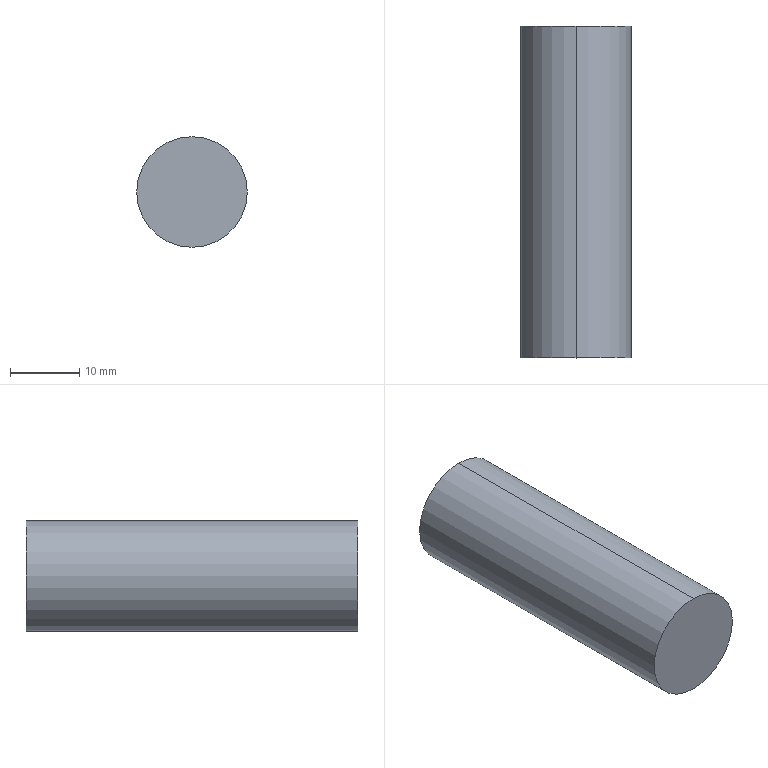Part | SolidWorks | features Extrusion 1, HoleWzd 1 | 1 solid | 8 faces | box 16 x 48 x 16 mm | volume 8682 mm3 | cylinder 4 | cone 2 | plane 2 | commonest cylinder face diameters 6.8 x2 16 x2
STEP:
#1=CARTESIAN_POINT('',(0.,22.,-3.4));
#2=VERTEX_POINT('',#1);
#3=CARTESIAN_POINT('',(0.,22.,3.4));
#4=VERTEX_POINT('',#3);
#5=CARTESIAN_POINT('',(0.,22.,0.));
#6=DIRECTION('',(0.,1.,0.));
#7=DIRECTION('',(0.,0.,1.));
#8=AXIS2_PLACEMENT_3D('',#5,#6,#7);
#9=CIRCLE('',#8,3.4);
#10=EDGE_CURVE('',#2,#4,#9,.T.);
#11=ORIENTED_EDGE('',*,*,#10,.F.);
#12=CARTESIAN_POINT('',(0.,48.,-3.4));
#13=VERTEX_POINT('',#12);
#14=CARTESIAN_POINT('',(0.,48.,-3.4));
#15=DIRECTION('',(0.,1.,0.));
#16=VECTOR('',#15,1000.);
#17=LINE('',#14,#16);
#18=EDGE_CURVE('',#2,#13,#17,.T.);
#19=ORIENTED_EDGE('',*,*,#18,.T.);
#20=CARTESIAN_POINT('',(0.,48.,3.4));
#21=VERTEX_POINT('',#20);
#22=CARTESIAN_POINT('',(0.,48.,0.));
#23=DIRECTION('',(0.,1.,0.));
#24=DIRECTION('',(0.,0.,1.));
#25=AXIS2_PLACEMENT_3D('',#22,#23,#24);
#26=CIRCLE('',#25,3.4);
#27=EDGE_CURVE('',#13,#21,#26,.T.);
#28=ORIENTED_EDGE('',*,*,#27,.T.);
#29=CARTESIAN_POINT('',(0.,48.,3.4));
#30=DIRECTION('',(0.,1.,0.));
#31=VECTOR('',#30,1000.);
#32=LINE('',#29,#31);
#33=EDGE_CURVE('',#4,#21,#32,.T.);
#34=ORIENTED_EDGE('',*,*,#33,.F.);
#35=EDGE_LOOP('',(#11,#19,#28,#34));
#36=FACE_OUTER_BOUND('',#35,.T.);
#37=CARTESIAN_POINT('',(0.,48.,0.));
#38=DIRECTION('',(0.,1.,0.));
#39=DIRECTION('',(0.,0.,1.));
#40=AXIS2_PLACEMENT_3D('',#37,#38,#39);
#41=CYLINDRICAL_SURFACE('',#40,3.4);
#42=ADVANCED_FACE('',(#36),#41,.F.);
#43=CARTESIAN_POINT('',(0.,19.957,0.));
#44=VERTEX_POINT('',#43);
#45=CARTESIAN_POINT('',(0.,22.,3.4));
#46=DIRECTION('',(0.,0.515,0.8572));
#47=VECTOR('',#46,1000.);
#48=LINE('',#45,#47);
#49=EDGE_CURVE('',#44,#4,#48,.T.);
#50=ORIENTED_EDGE('',*,*,#49,.F.);
#51=CARTESIAN_POINT('',(0.,22.,-3.4));
#52=DIRECTION('',(0.,0.515,-0.8572));
#53=VECTOR('',#52,1000.);
#54=LINE('',#51,#53);
#55=EDGE_CURVE('',#44,#2,#54,.T.);
#56=ORIENTED_EDGE('',*,*,#55,.T.);
#57=ORIENTED_EDGE('',*,*,#10,.T.);
#58=EDGE_LOOP('',(#50,#56,#57));
#59=FACE_OUTER_BOUND('',#58,.T.);
#60=CARTESIAN_POINT('',(0.,22.,0.));
#61=DIRECTION('',(0.,1.,0.));
#62=DIRECTION('',(0.,0.,1.));
#63=AXIS2_PLACEMENT_3D('',#60,#61,#62);
#64=CONICAL_SURFACE('',#63,3.4,1.03);
#65=ADVANCED_FACE('',(#59),#64,.F.);
#66=CARTESIAN_POINT('',(0.,48.,8.));
#67=VERTEX_POINT('',#66);
#68=CARTESIAN_POINT('',(0.,48.,-8.));
#69=VERTEX_POINT('',#68);
#70=CARTESIAN_POINT('',(0.,48.,0.));
#71=DIRECTION('',(0.,1.,0.));
#72=DIRECTION('',(0.,0.,1.));
#73=AXIS2_PLACEMENT_3D('',#70,#71,#72);
#74=CIRCLE('',#73,8.);
#75=EDGE_CURVE('',#67,#69,#74,.T.);
#76=ORIENTED_EDGE('',*,*,#75,.F.);
#77=CARTESIAN_POINT('',(0.,0.,8.));
#78=VERTEX_POINT('',#77);
#79=CARTESIAN_POINT('',(0.,48.,8.));
#80=DIRECTION('',(0.,-1.,0.));
#81=VECTOR('',#80,1000.);
#82=LINE('',#79,#81);
#83=EDGE_CURVE('',#67,#78,#82,.T.);
#84=ORIENTED_EDGE('',*,*,#83,.T.);
#85=CARTESIAN_POINT('',(0.,0.,-8.));
#86=VERTEX_POINT('',#85);
#87=CARTESIAN_POINT('',(0.,0.,0.));
#88=DIRECTION('',(0.,1.,0.));
#89=DIRECTION('',(0.,0.,1.));
#90=AXIS2_PLACEMENT_3D('',#87,#88,#89);
#91=CIRCLE('',#90,8.);
#92=EDGE_CURVE('',#78,#86,#91,.T.);
#93=ORIENTED_EDGE('',*,*,#92,.T.);
#94=CARTESIAN_POINT('',(0.,48.,-8.));
#95=DIRECTION('',(0.,-1.,0.));
#96=VECTOR('',#95,1000.);
#97=LINE('',#94,#96);
#98=EDGE_CURVE('',#69,#86,#97,.T.);
#99=ORIENTED_EDGE('',*,*,#98,.F.);
#100=EDGE_LOOP('',(#76,#84,#93,#99));
#101=FACE_OUTER_BOUND('',#100,.T.);
#102=CARTESIAN_POINT('',(0.,48.,0.));
#103=DIRECTION('',(0.,-1.,0.));
#104=DIRECTION('',(0.,0.,-1.));
#105=AXIS2_PLACEMENT_3D('',#102,#103,#104);
#106=CYLINDRICAL_SURFACE('',#105,8.);
#107=ADVANCED_FACE('',(#101),#106,.T.);
#108=ORIENTED_EDGE('',*,*,#83,.F.);
#109=CARTESIAN_POINT('',(0.,48.,0.));
#110=DIRECTION('',(0.,1.,0.));
#111=DIRECTION('',(0.,0.,1.));
#112=AXIS2_PLACEMENT_3D('',#109,#110,#111);
#113=CIRCLE('',#112,8.);
#114=EDGE_CURVE('',#69,#67,#113,.T.);
#115=ORIENTED_EDGE('',*,*,#114,.F.);
#116=ORIENTED_EDGE('',*,*,#98,.T.);
#117=CARTESIAN_POINT('',(0.,0.,0.));
#118=DIRECTION('',(0.,1.,0.));
#119=DIRECTION('',(0.,0.,1.));
#120=AXIS2_PLACEMENT_3D('',#117,#118,#119);
#121=CIRCLE('',#120,8.);
#122=EDGE_CURVE('',#86,#78,#121,.T.);
#123=ORIENTED_EDGE('',*,*,#122,.T.);
#124=EDGE_LOOP('',(#108,#115,#116,#123));
#125=FACE_OUTER_BOUND('',#124,.T.);
#126=CARTESIAN_POINT('',(0.,48.,0.));
#127=DIRECTION('',(0.,-1.,0.));
#128=DIRECTION('',(0.,0.,-1.));
#129=AXIS2_PLACEMENT_3D('',#126,#127,#128);
#130=CYLINDRICAL_SURFACE('',#129,8.);
#131=ADVANCED_FACE('',(#125),#130,.T.);
#132=CARTESIAN_POINT('',(0.,48.,0.));
#133=DIRECTION('',(0.,1.,0.));
#134=DIRECTION('',(0.,0.,1.));
#135=AXIS2_PLACEMENT_3D('',#132,#133,#134);
#136=CIRCLE('',#135,3.4);
#137=EDGE_CURVE('',#21,#13,#136,.T.);
#138=ORIENTED_EDGE('',*,*,#137,.F.);
#139=ORIENTED_EDGE('',*,*,#27,.F.);
#140=EDGE_LOOP('',(#138,#139));
#141=FACE_BOUND('',#140,.T.);
#142=ORIENTED_EDGE('',*,*,#114,.T.);
#143=ORIENTED_EDGE('',*,*,#75,.T.);
#144=EDGE_LOOP('',(#142,#143));
#145=FACE_OUTER_BOUND('',#144,.T.);
#146=CARTESIAN_POINT('',(0.,48.,0.));
#147=DIRECTION('',(0.,1.,0.));
#148=DIRECTION('',(0.,0.,1.));
#149=AXIS2_PLACEMENT_3D('',#146,#147,#148);
#150=PLANE('',#149);
#151=ADVANCED_FACE('',(#141,#145),#150,.T.);
#152=ORIENTED_EDGE('',*,*,#122,.F.);
#153=ORIENTED_EDGE('',*,*,#92,.F.);
#154=EDGE_LOOP('',(#152,#153));
#155=FACE_OUTER_BOUND('',#154,.T.);
#156=CARTESIAN_POINT('',(0.,0.,0.));
#157=DIRECTION('',(0.,1.,0.));
#158=DIRECTION('',(0.,0.,1.));
#159=AXIS2_PLACEMENT_3D('',#156,#157,#158);
#160=PLANE('',#159);
#161=ADVANCED_FACE('',(#155),#160,.F.);
#162=ORIENTED_EDGE('',*,*,#55,.F.);
#163=ORIENTED_EDGE('',*,*,#49,.T.);
#164=CARTESIAN_POINT('',(0.,22.,0.));
#165=DIRECTION('',(0.,1.,0.));
#166=DIRECTION('',(0.,0.,1.));
#167=AXIS2_PLACEMENT_3D('',#164,#165,#166);
#168=CIRCLE('',#167,3.4);
#169=EDGE_CURVE('',#4,#2,#168,.T.);
#170=ORIENTED_EDGE('',*,*,#169,.T.);
#171=EDGE_LOOP('',(#162,#163,#170));
#172=FACE_OUTER_BOUND('',#171,.T.);
#173=CARTESIAN_POINT('',(0.,22.,0.));
#174=DIRECTION('',(0.,1.,0.));
#175=DIRECTION('',(0.,0.,1.));
#176=AXIS2_PLACEMENT_3D('',#173,#174,#175);
#177=CONICAL_SURFACE('',#176,3.4,1.03);
#178=ADVANCED_FACE('',(#172),#177,.F.);
#179=ORIENTED_EDGE('',*,*,#18,.F.);
#180=ORIENTED_EDGE('',*,*,#169,.F.);
#181=ORIENTED_EDGE('',*,*,#33,.T.);
#182=ORIENTED_EDGE('',*,*,#137,.T.);
#183=EDGE_LOOP('',(#179,#180,#181,#182));
#184=FACE_OUTER_BOUND('',#183,.T.);
#185=CARTESIAN_POINT('',(0.,48.,0.));
#186=DIRECTION('',(0.,1.,0.));
#187=DIRECTION('',(0.,0.,1.));
#188=AXIS2_PLACEMENT_3D('',#185,#186,#187);
#189=CYLINDRICAL_SURFACE('',#188,3.4);
#190=ADVANCED_FACE('',(#184),#189,.F.);
#191=CLOSED_SHELL('',(#42,#65,#107,#131,#151,#161,#178,#190));
#192=MANIFOLD_SOLID_BREP('',#191);
#193=CARTESIAN_POINT('',(0.,0.,0.));
#194=DIRECTION('',(0.,0.,1.));
#195=DIRECTION('',(1.,0.,0.));
#196=AXIS2_PLACEMENT_3D('',#193,#194,#195);
#197=(LENGTH_UNIT()NAMED_UNIT(*)SI_UNIT(.MILLI.,.METRE.));
#198=UNCERTAINTY_MEASURE_WITH_UNIT(LENGTH_MEASURE(0.00001),#197,'','');
#199=(NAMED_UNIT(*)PLANE_ANGLE_UNIT()SI_UNIT($,.RADIAN.));
#200=(NAMED_UNIT(*)SI_UNIT($,.STERADIAN.)SOLID_ANGLE_UNIT());
#201=(GEOMETRIC_REPRESENTATION_CONTEXT(3)GLOBAL_UNCERTAINTY_ASSIGNED_CONTEXT((#198))GLOBAL_UNIT_ASSIGNED_CONTEXT((#197,#199,#200))REPRESENTATION_CONTEXT('',''));
#202=ADVANCED_BREP_SHAPE_REPRESENTATION('',(#192,#196),#201);